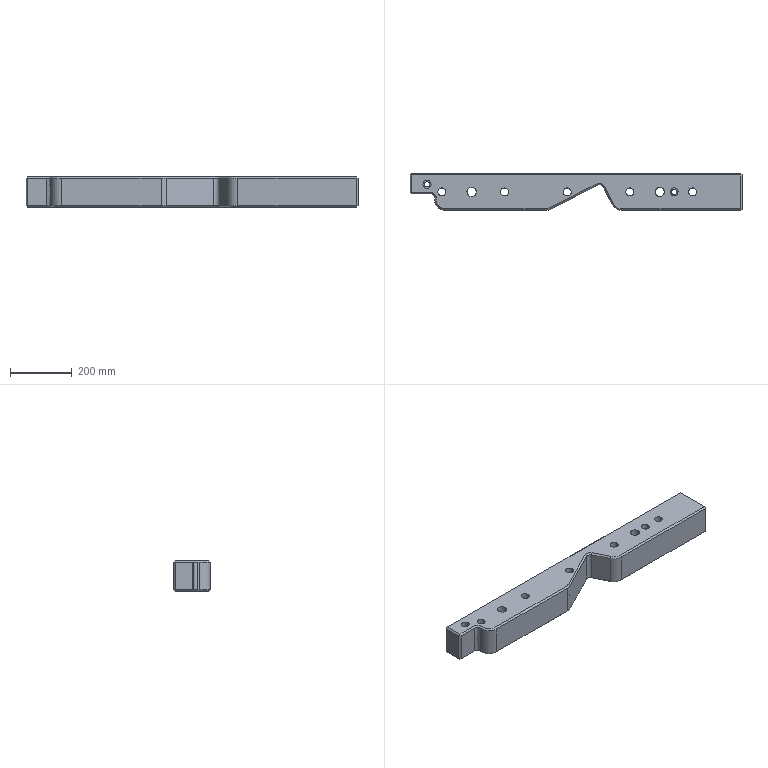Part | STEP file | solid 108 | 1 solid | 69 faces | box 1075 x 120.001 x 100 mm | volume 10949894 mm3 | plane 27 | spline 25 | cylinder 15 | other 2 | commonest cylinder face diameters 26 x8 70 x3 17.5 x2 30 x2